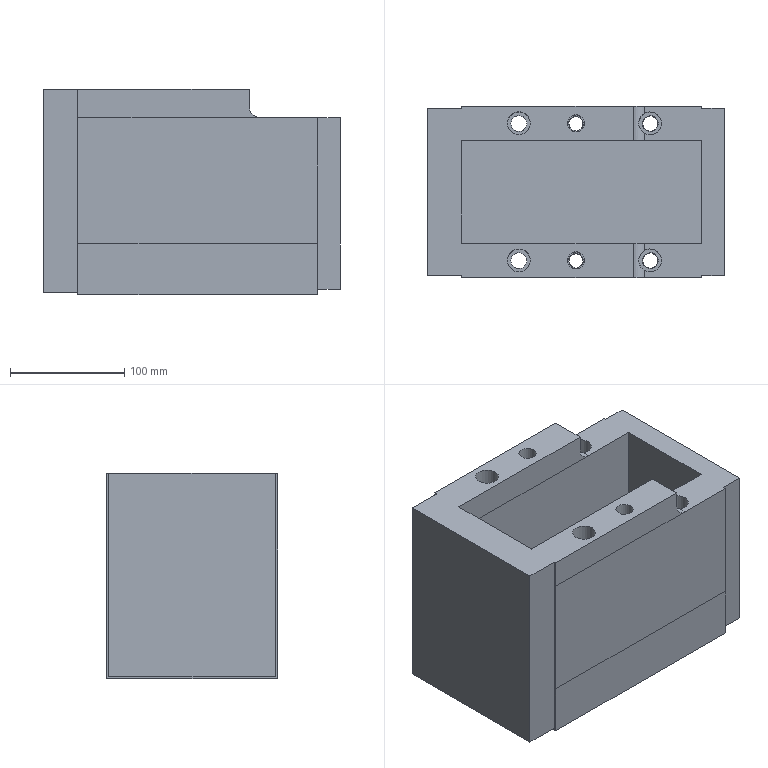Part | NX | features MAIN_BODY 2 | 1 solid | 53 faces | box 260 x 150 x 180 mm | volume 4007747 mm3 | plane 29 | cylinder 14 | spline 10 | commonest cylinder face diameters 20 x6 14 x4 13 x2 15 x2